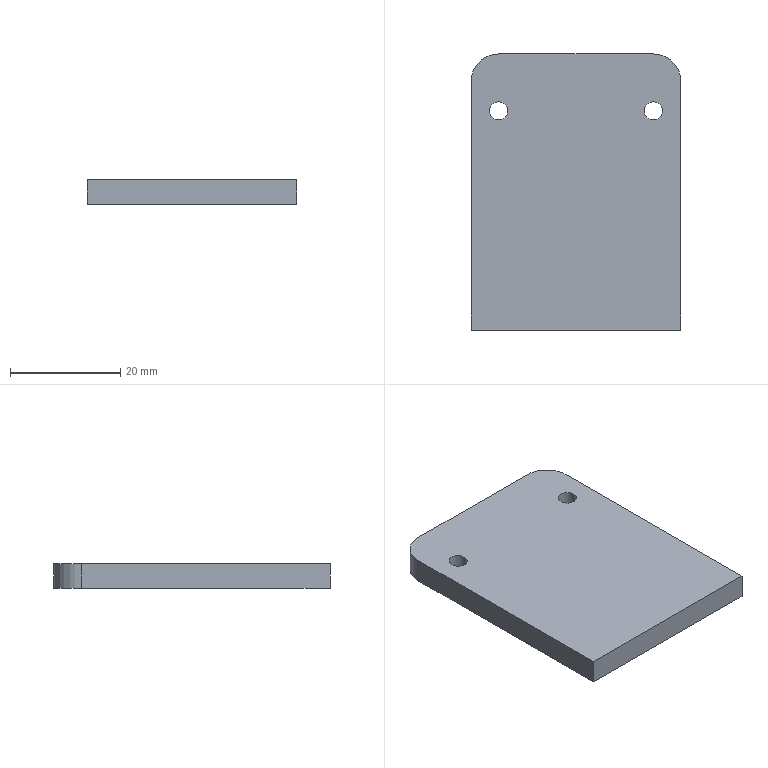Part | SolidWorks | features FlatPattern 1, HoleWzd 1, SMBaseFlange 1, SheetMetal 1 | 1 solid | 12 faces | box 38 x 50 x 4.5 mm | volume 8425 mm3 | cylinder 6 | plane 6 | commonest cylinder face diameters 3.3 x4 10 x2
STEP:
#1=CARTESIAN_POINT('',(-15.65,14.7,0.));
#2=VERTEX_POINT('',#1);
#3=CARTESIAN_POINT('',(-12.35,14.7,0.));
#4=VERTEX_POINT('',#3);
#5=CARTESIAN_POINT('',(-14.,14.7,0.));
#6=DIRECTION('',(0.,0.,1.));
#7=DIRECTION('',(1.,0.,0.));
#8=AXIS2_PLACEMENT_3D('',#5,#6,#7);
#9=CIRCLE('',#8,1.65);
#10=EDGE_CURVE('',#2,#4,#9,.T.);
#11=ORIENTED_EDGE('',*,*,#10,.F.);
#12=CARTESIAN_POINT('',(-15.65,14.7,4.5));
#13=VERTEX_POINT('',#12);
#14=CARTESIAN_POINT('',(-15.65,14.7,4.5));
#15=DIRECTION('',(0.,0.,1.));
#16=VECTOR('',#15,1000.);
#17=LINE('',#14,#16);
#18=EDGE_CURVE('',#2,#13,#17,.T.);
#19=ORIENTED_EDGE('',*,*,#18,.T.);
#20=CARTESIAN_POINT('',(-12.35,14.7,4.5));
#21=VERTEX_POINT('',#20);
#22=CARTESIAN_POINT('',(-14.,14.7,4.5));
#23=DIRECTION('',(0.,0.,1.));
#24=DIRECTION('',(1.,0.,0.));
#25=AXIS2_PLACEMENT_3D('',#22,#23,#24);
#26=CIRCLE('',#25,1.65);
#27=EDGE_CURVE('',#13,#21,#26,.T.);
#28=ORIENTED_EDGE('',*,*,#27,.T.);
#29=CARTESIAN_POINT('',(-12.35,14.7,4.5));
#30=DIRECTION('',(0.,0.,1.));
#31=VECTOR('',#30,1000.);
#32=LINE('',#29,#31);
#33=EDGE_CURVE('',#4,#21,#32,.T.);
#34=ORIENTED_EDGE('',*,*,#33,.F.);
#35=EDGE_LOOP('',(#11,#19,#28,#34));
#36=FACE_OUTER_BOUND('',#35,.T.);
#37=CARTESIAN_POINT('',(-14.,14.7,4.5));
#38=DIRECTION('',(0.,0.,1.));
#39=DIRECTION('',(1.,0.,0.));
#40=AXIS2_PLACEMENT_3D('',#37,#38,#39);
#41=CYLINDRICAL_SURFACE('',#40,1.65);
#42=ADVANCED_FACE('',(#36),#41,.F.);
#43=CARTESIAN_POINT('',(12.35,14.7,0.));
#44=VERTEX_POINT('',#43);
#45=CARTESIAN_POINT('',(15.65,14.7,0.));
#46=VERTEX_POINT('',#45);
#47=CARTESIAN_POINT('',(14.,14.7,0.));
#48=DIRECTION('',(0.,0.,1.));
#49=DIRECTION('',(1.,0.,0.));
#50=AXIS2_PLACEMENT_3D('',#47,#48,#49);
#51=CIRCLE('',#50,1.65);
#52=EDGE_CURVE('',#44,#46,#51,.T.);
#53=ORIENTED_EDGE('',*,*,#52,.F.);
#54=CARTESIAN_POINT('',(12.35,14.7,4.5));
#55=VERTEX_POINT('',#54);
#56=CARTESIAN_POINT('',(12.35,14.7,4.5));
#57=DIRECTION('',(0.,0.,1.));
#58=VECTOR('',#57,1000.);
#59=LINE('',#56,#58);
#60=EDGE_CURVE('',#44,#55,#59,.T.);
#61=ORIENTED_EDGE('',*,*,#60,.T.);
#62=CARTESIAN_POINT('',(15.65,14.7,4.5));
#63=VERTEX_POINT('',#62);
#64=CARTESIAN_POINT('',(14.,14.7,4.5));
#65=DIRECTION('',(0.,0.,1.));
#66=DIRECTION('',(1.,0.,0.));
#67=AXIS2_PLACEMENT_3D('',#64,#65,#66);
#68=CIRCLE('',#67,1.65);
#69=EDGE_CURVE('',#55,#63,#68,.T.);
#70=ORIENTED_EDGE('',*,*,#69,.T.);
#71=CARTESIAN_POINT('',(15.65,14.7,4.5));
#72=DIRECTION('',(0.,0.,1.));
#73=VECTOR('',#72,1000.);
#74=LINE('',#71,#73);
#75=EDGE_CURVE('',#46,#63,#74,.T.);
#76=ORIENTED_EDGE('',*,*,#75,.F.);
#77=EDGE_LOOP('',(#53,#61,#70,#76));
#78=FACE_OUTER_BOUND('',#77,.T.);
#79=CARTESIAN_POINT('',(14.,14.7,4.5));
#80=DIRECTION('',(0.,0.,1.));
#81=DIRECTION('',(1.,0.,0.));
#82=AXIS2_PLACEMENT_3D('',#79,#80,#81);
#83=CYLINDRICAL_SURFACE('',#82,1.65);
#84=ADVANCED_FACE('',(#78),#83,.F.);
#85=CARTESIAN_POINT('',(-14.,14.7,4.5));
#86=DIRECTION('',(0.,0.,1.));
#87=DIRECTION('',(1.,0.,0.));
#88=AXIS2_PLACEMENT_3D('',#85,#86,#87);
#89=CIRCLE('',#88,1.65);
#90=EDGE_CURVE('',#21,#13,#89,.T.);
#91=ORIENTED_EDGE('',*,*,#90,.F.);
#92=ORIENTED_EDGE('',*,*,#27,.F.);
#93=EDGE_LOOP('',(#91,#92));
#94=FACE_BOUND('',#93,.T.);
#95=CARTESIAN_POINT('',(14.,14.7,4.5));
#96=DIRECTION('',(0.,0.,1.));
#97=DIRECTION('',(1.,0.,0.));
#98=AXIS2_PLACEMENT_3D('',#95,#96,#97);
#99=CIRCLE('',#98,1.65);
#100=EDGE_CURVE('',#63,#55,#99,.T.);
#101=ORIENTED_EDGE('',*,*,#100,.F.);
#102=ORIENTED_EDGE('',*,*,#69,.F.);
#103=EDGE_LOOP('',(#101,#102));
#104=FACE_BOUND('',#103,.T.);
#105=CARTESIAN_POINT('',(19.,-25.,4.5));
#106=VERTEX_POINT('',#105);
#107=CARTESIAN_POINT('',(19.,20.,4.5));
#108=VERTEX_POINT('',#107);
#109=CARTESIAN_POINT('',(19.,20.,4.5));
#110=DIRECTION('',(0.,1.,0.));
#111=VECTOR('',#110,1000.);
#112=LINE('',#109,#111);
#113=EDGE_CURVE('',#106,#108,#112,.T.);
#114=ORIENTED_EDGE('',*,*,#113,.T.);
#115=CARTESIAN_POINT('',(14.,25.,4.5));
#116=VERTEX_POINT('',#115);
#117=CARTESIAN_POINT('',(14.,20.,4.5));
#118=DIRECTION('',(0.,0.,1.));
#119=DIRECTION('',(-1.,0.,0.));
#120=AXIS2_PLACEMENT_3D('',#117,#118,#119);
#121=CIRCLE('',#120,5.);
#122=EDGE_CURVE('',#108,#116,#121,.T.);
#123=ORIENTED_EDGE('',*,*,#122,.T.);
#124=CARTESIAN_POINT('',(-14.,25.,4.5));
#125=VERTEX_POINT('',#124);
#126=CARTESIAN_POINT('',(-14.,25.,4.5));
#127=DIRECTION('',(-1.,0.,0.));
#128=VECTOR('',#127,1000.);
#129=LINE('',#126,#128);
#130=EDGE_CURVE('',#116,#125,#129,.T.);
#131=ORIENTED_EDGE('',*,*,#130,.T.);
#132=CARTESIAN_POINT('',(-19.,20.,4.5));
#133=VERTEX_POINT('',#132);
#134=CARTESIAN_POINT('',(-14.,20.,4.5));
#135=DIRECTION('',(0.,0.,1.));
#136=DIRECTION('',(1.,0.,0.));
#137=AXIS2_PLACEMENT_3D('',#134,#135,#136);
#138=CIRCLE('',#137,5.);
#139=EDGE_CURVE('',#125,#133,#138,.T.);
#140=ORIENTED_EDGE('',*,*,#139,.T.);
#141=CARTESIAN_POINT('',(-19.,-25.,4.5));
#142=VERTEX_POINT('',#141);
#143=CARTESIAN_POINT('',(-19.,20.,4.5));
#144=DIRECTION('',(0.,-1.,0.));
#145=VECTOR('',#144,1000.);
#146=LINE('',#143,#145);
#147=EDGE_CURVE('',#133,#142,#146,.T.);
#148=ORIENTED_EDGE('',*,*,#147,.T.);
#149=CARTESIAN_POINT('',(-19.,-25.,4.5));
#150=DIRECTION('',(1.,0.,0.));
#151=VECTOR('',#150,1000.);
#152=LINE('',#149,#151);
#153=EDGE_CURVE('',#142,#106,#152,.T.);
#154=ORIENTED_EDGE('',*,*,#153,.T.);
#155=EDGE_LOOP('',(#114,#123,#131,#140,#148,#154));
#156=FACE_OUTER_BOUND('',#155,.T.);
#157=CARTESIAN_POINT('',(-14.,20.,4.5));
#158=DIRECTION('',(0.,0.,1.));
#159=DIRECTION('',(1.,0.,0.));
#160=AXIS2_PLACEMENT_3D('',#157,#158,#159);
#161=PLANE('',#160);
#162=ADVANCED_FACE('',(#94,#104,#156),#161,.T.);
#163=CARTESIAN_POINT('',(-14.,14.7,0.));
#164=DIRECTION('',(0.,0.,1.));
#165=DIRECTION('',(1.,0.,0.));
#166=AXIS2_PLACEMENT_3D('',#163,#164,#165);
#167=CIRCLE('',#166,1.65);
#168=EDGE_CURVE('',#4,#2,#167,.T.);
#169=ORIENTED_EDGE('',*,*,#168,.T.);
#170=ORIENTED_EDGE('',*,*,#10,.T.);
#171=EDGE_LOOP('',(#169,#170));
#172=FACE_BOUND('',#171,.T.);
#173=CARTESIAN_POINT('',(14.,14.7,0.));
#174=DIRECTION('',(0.,0.,1.));
#175=DIRECTION('',(1.,0.,0.));
#176=AXIS2_PLACEMENT_3D('',#173,#174,#175);
#177=CIRCLE('',#176,1.65);
#178=EDGE_CURVE('',#46,#44,#177,.T.);
#179=ORIENTED_EDGE('',*,*,#178,.T.);
#180=ORIENTED_EDGE('',*,*,#52,.T.);
#181=EDGE_LOOP('',(#179,#180));
#182=FACE_BOUND('',#181,.T.);
#183=CARTESIAN_POINT('',(19.,-25.,0.));
#184=VERTEX_POINT('',#183);
#185=CARTESIAN_POINT('',(19.,20.,0.));
#186=VERTEX_POINT('',#185);
#187=CARTESIAN_POINT('',(19.,20.,0.));
#188=DIRECTION('',(0.,1.,0.));
#189=VECTOR('',#188,1000.);
#190=LINE('',#187,#189);
#191=EDGE_CURVE('',#184,#186,#190,.T.);
#192=ORIENTED_EDGE('',*,*,#191,.F.);
#193=CARTESIAN_POINT('',(-19.,-25.,0.));
#194=VERTEX_POINT('',#193);
#195=CARTESIAN_POINT('',(-19.,-25.,0.));
#196=DIRECTION('',(1.,0.,0.));
#197=VECTOR('',#196,1000.);
#198=LINE('',#195,#197);
#199=EDGE_CURVE('',#194,#184,#198,.T.);
#200=ORIENTED_EDGE('',*,*,#199,.F.);
#201=CARTESIAN_POINT('',(-19.,20.,0.));
#202=VERTEX_POINT('',#201);
#203=CARTESIAN_POINT('',(-19.,20.,0.));
#204=DIRECTION('',(0.,-1.,0.));
#205=VECTOR('',#204,1000.);
#206=LINE('',#203,#205);
#207=EDGE_CURVE('',#202,#194,#206,.T.);
#208=ORIENTED_EDGE('',*,*,#207,.F.);
#209=CARTESIAN_POINT('',(-14.,25.,0.));
#210=VERTEX_POINT('',#209);
#211=CARTESIAN_POINT('',(-14.,20.,0.));
#212=DIRECTION('',(0.,0.,1.));
#213=DIRECTION('',(1.,0.,0.));
#214=AXIS2_PLACEMENT_3D('',#211,#212,#213);
#215=CIRCLE('',#214,5.);
#216=EDGE_CURVE('',#210,#202,#215,.T.);
#217=ORIENTED_EDGE('',*,*,#216,.F.);
#218=CARTESIAN_POINT('',(14.,25.,0.));
#219=VERTEX_POINT('',#218);
#220=CARTESIAN_POINT('',(-14.,25.,0.));
#221=DIRECTION('',(-1.,0.,0.));
#222=VECTOR('',#221,1000.);
#223=LINE('',#220,#222);
#224=EDGE_CURVE('',#219,#210,#223,.T.);
#225=ORIENTED_EDGE('',*,*,#224,.F.);
#226=CARTESIAN_POINT('',(14.,20.,0.));
#227=DIRECTION('',(0.,0.,1.));
#228=DIRECTION('',(-1.,0.,0.));
#229=AXIS2_PLACEMENT_3D('',#226,#227,#228);
#230=CIRCLE('',#229,5.);
#231=EDGE_CURVE('',#186,#219,#230,.T.);
#232=ORIENTED_EDGE('',*,*,#231,.F.);
#233=EDGE_LOOP('',(#192,#200,#208,#217,#225,#232));
#234=FACE_OUTER_BOUND('',#233,.T.);
#235=CARTESIAN_POINT('',(-14.,20.,0.));
#236=DIRECTION('',(0.,0.,1.));
#237=DIRECTION('',(1.,0.,0.));
#238=AXIS2_PLACEMENT_3D('',#235,#236,#237);
#239=PLANE('',#238);
#240=ADVANCED_FACE('',(#172,#182,#234),#239,.F.);
#241=ORIENTED_EDGE('',*,*,#191,.T.);
#242=CARTESIAN_POINT('',(19.,20.,4.5));
#243=DIRECTION('',(0.,0.,-1.));
#244=VECTOR('',#243,1000.);
#245=LINE('',#242,#244);
#246=EDGE_CURVE('',#108,#186,#245,.T.);
#247=ORIENTED_EDGE('',*,*,#246,.F.);
#248=ORIENTED_EDGE('',*,*,#113,.F.);
#249=CARTESIAN_POINT('',(19.,-25.,4.5));
#250=DIRECTION('',(0.,0.,-1.));
#251=VECTOR('',#250,1000.);
#252=LINE('',#249,#251);
#253=EDGE_CURVE('',#106,#184,#252,.T.);
#254=ORIENTED_EDGE('',*,*,#253,.T.);
#255=EDGE_LOOP('',(#241,#247,#248,#254));
#256=FACE_OUTER_BOUND('',#255,.T.);
#257=CARTESIAN_POINT('',(19.,20.,4.5));
#258=DIRECTION('',(-1.,0.,0.));
#259=DIRECTION('',(0.,-1.,0.));
#260=AXIS2_PLACEMENT_3D('',#257,#258,#259);
#261=PLANE('',#260);
#262=ADVANCED_FACE('',(#256),#261,.F.);
#263=ORIENTED_EDGE('',*,*,#231,.T.);
#264=CARTESIAN_POINT('',(14.,25.,4.5));
#265=DIRECTION('',(0.,0.,-1.));
#266=VECTOR('',#265,1000.);
#267=LINE('',#264,#266);
#268=EDGE_CURVE('',#116,#219,#267,.T.);
#269=ORIENTED_EDGE('',*,*,#268,.F.);
#270=ORIENTED_EDGE('',*,*,#122,.F.);
#271=ORIENTED_EDGE('',*,*,#246,.T.);
#272=EDGE_LOOP('',(#263,#269,#270,#271));
#273=FACE_OUTER_BOUND('',#272,.T.);
#274=CARTESIAN_POINT('',(14.,20.,4.5));
#275=DIRECTION('',(0.,0.,-1.));
#276=DIRECTION('',(-1.,0.,0.));
#277=AXIS2_PLACEMENT_3D('',#274,#275,#276);
#278=CYLINDRICAL_SURFACE('',#277,5.);
#279=ADVANCED_FACE('',(#273),#278,.T.);
#280=ORIENTED_EDGE('',*,*,#224,.T.);
#281=CARTESIAN_POINT('',(-14.,25.,4.5));
#282=DIRECTION('',(0.,0.,-1.));
#283=VECTOR('',#282,1000.);
#284=LINE('',#281,#283);
#285=EDGE_CURVE('',#125,#210,#284,.T.);
#286=ORIENTED_EDGE('',*,*,#285,.F.);
#287=ORIENTED_EDGE('',*,*,#130,.F.);
#288=ORIENTED_EDGE('',*,*,#268,.T.);
#289=EDGE_LOOP('',(#280,#286,#287,#288));
#290=FACE_OUTER_BOUND('',#289,.T.);
#291=CARTESIAN_POINT('',(-14.,25.,4.5));
#292=DIRECTION('',(0.,-1.,0.));
#293=DIRECTION('',(0.,0.,-1.));
#294=AXIS2_PLACEMENT_3D('',#291,#292,#293);
#295=PLANE('',#294);
#296=ADVANCED_FACE('',(#290),#295,.F.);
#297=ORIENTED_EDGE('',*,*,#216,.T.);
#298=CARTESIAN_POINT('',(-19.,20.,4.5));
#299=DIRECTION('',(0.,0.,-1.));
#300=VECTOR('',#299,1000.);
#301=LINE('',#298,#300);
#302=EDGE_CURVE('',#133,#202,#301,.T.);
#303=ORIENTED_EDGE('',*,*,#302,.F.);
#304=ORIENTED_EDGE('',*,*,#139,.F.);
#305=ORIENTED_EDGE('',*,*,#285,.T.);
#306=EDGE_LOOP('',(#297,#303,#304,#305));
#307=FACE_OUTER_BOUND('',#306,.T.);
#308=CARTESIAN_POINT('',(-14.,20.,4.5));
#309=DIRECTION('',(0.,0.,-1.));
#310=DIRECTION('',(-1.,0.,0.));
#311=AXIS2_PLACEMENT_3D('',#308,#309,#310);
#312=CYLINDRICAL_SURFACE('',#311,5.);
#313=ADVANCED_FACE('',(#307),#312,.T.);
#314=ORIENTED_EDGE('',*,*,#207,.T.);
#315=CARTESIAN_POINT('',(-19.,-25.,4.5));
#316=DIRECTION('',(0.,0.,-1.));
#317=VECTOR('',#316,1000.);
#318=LINE('',#315,#317);
#319=EDGE_CURVE('',#142,#194,#318,.T.);
#320=ORIENTED_EDGE('',*,*,#319,.F.);
#321=ORIENTED_EDGE('',*,*,#147,.F.);
#322=ORIENTED_EDGE('',*,*,#302,.T.);
#323=EDGE_LOOP('',(#314,#320,#321,#322));
#324=FACE_OUTER_BOUND('',#323,.T.);
#325=CARTESIAN_POINT('',(-19.,20.,4.5));
#326=DIRECTION('',(1.,0.,0.));
#327=DIRECTION('',(0.,1.,0.));
#328=AXIS2_PLACEMENT_3D('',#325,#326,#327);
#329=PLANE('',#328);
#330=ADVANCED_FACE('',(#324),#329,.F.);
#331=ORIENTED_EDGE('',*,*,#199,.T.);
#332=ORIENTED_EDGE('',*,*,#253,.F.);
#333=ORIENTED_EDGE('',*,*,#153,.F.);
#334=ORIENTED_EDGE('',*,*,#319,.T.);
#335=EDGE_LOOP('',(#331,#332,#333,#334));
#336=FACE_OUTER_BOUND('',#335,.T.);
#337=CARTESIAN_POINT('',(-19.,-25.,4.5));
#338=DIRECTION('',(0.,1.,0.));
#339=DIRECTION('',(0.,0.,1.));
#340=AXIS2_PLACEMENT_3D('',#337,#338,#339);
#341=PLANE('',#340);
#342=ADVANCED_FACE('',(#336),#341,.F.);
#343=ORIENTED_EDGE('',*,*,#60,.F.);
#344=ORIENTED_EDGE('',*,*,#178,.F.);
#345=ORIENTED_EDGE('',*,*,#75,.T.);
#346=ORIENTED_EDGE('',*,*,#100,.T.);
#347=EDGE_LOOP('',(#343,#344,#345,#346));
#348=FACE_OUTER_BOUND('',#347,.T.);
#349=CARTESIAN_POINT('',(14.,14.7,4.5));
#350=DIRECTION('',(0.,0.,1.));
#351=DIRECTION('',(1.,0.,0.));
#352=AXIS2_PLACEMENT_3D('',#349,#350,#351);
#353=CYLINDRICAL_SURFACE('',#352,1.65);
#354=ADVANCED_FACE('',(#348),#353,.F.);
#355=ORIENTED_EDGE('',*,*,#18,.F.);
#356=ORIENTED_EDGE('',*,*,#168,.F.);
#357=ORIENTED_EDGE('',*,*,#33,.T.);
#358=ORIENTED_EDGE('',*,*,#90,.T.);
#359=EDGE_LOOP('',(#355,#356,#357,#358));
#360=FACE_OUTER_BOUND('',#359,.T.);
#361=CARTESIAN_POINT('',(-14.,14.7,4.5));
#362=DIRECTION('',(0.,0.,1.));
#363=DIRECTION('',(1.,0.,0.));
#364=AXIS2_PLACEMENT_3D('',#361,#362,#363);
#365=CYLINDRICAL_SURFACE('',#364,1.65);
#366=ADVANCED_FACE('',(#360),#365,.F.);
#367=CLOSED_SHELL('',(#42,#84,#162,#240,#262,#279,#296,#313,#330,#342,#354,#366));
#368=MANIFOLD_SOLID_BREP('',#367);
#369=CARTESIAN_POINT('',(0.,0.,0.));
#370=DIRECTION('',(0.,0.,1.));
#371=DIRECTION('',(1.,0.,0.));
#372=AXIS2_PLACEMENT_3D('',#369,#370,#371);
#373=(LENGTH_UNIT()NAMED_UNIT(*)SI_UNIT(.MILLI.,.METRE.));
#374=UNCERTAINTY_MEASURE_WITH_UNIT(LENGTH_MEASURE(0.00001),#373,'','');
#375=(NAMED_UNIT(*)PLANE_ANGLE_UNIT()SI_UNIT($,.RADIAN.));
#376=(NAMED_UNIT(*)SI_UNIT($,.STERADIAN.)SOLID_ANGLE_UNIT());
#377=(GEOMETRIC_REPRESENTATION_CONTEXT(3)GLOBAL_UNCERTAINTY_ASSIGNED_CONTEXT((#374))GLOBAL_UNIT_ASSIGNED_CONTEXT((#373,#375,#376))REPRESENTATION_CONTEXT('',''));
#378=ADVANCED_BREP_SHAPE_REPRESENTATION('',(#368,#372),#377);